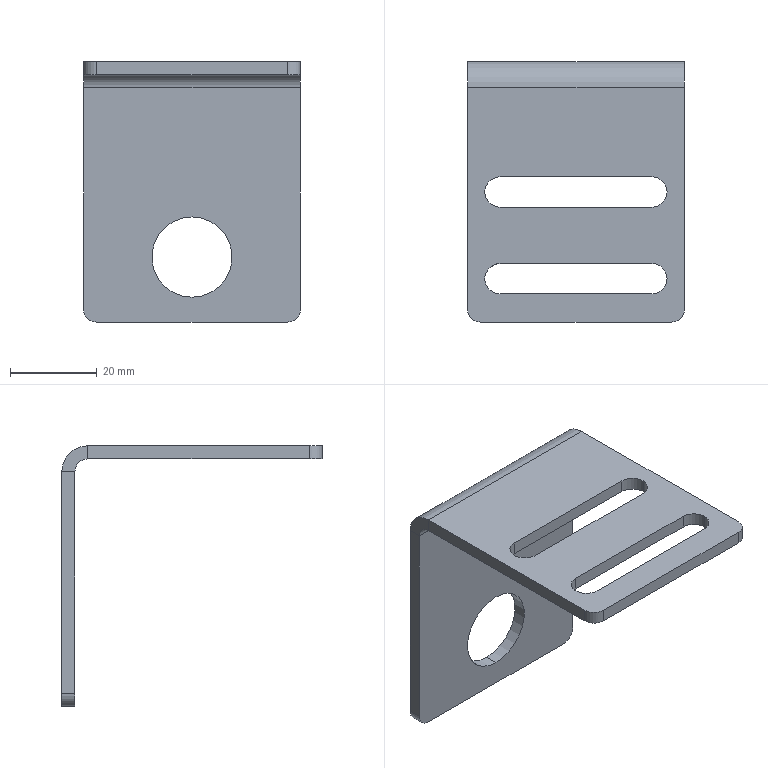Part | SolidWorks | features ICE 2, EdgeFlange 1, Fillet 1, FlatPattern 1, SMBaseFlange 1, SheetMetal 1 | 1 solid | 30 faces | box 50 x 60 x 60 mm | volume 14730 mm3 | plane 16 | cylinder 14 | commonest cylinder face diameters 7 x6 6 x5 18.5 x2 12 x1
STEP:
#1=CARTESIAN_POINT('',(0.,27.,-54.25));
#2=VERTEX_POINT('',#1);
#3=CARTESIAN_POINT('',(0.,27.,-35.75));
#4=VERTEX_POINT('',#3);
#5=CARTESIAN_POINT('',(0.,27.,-45.));
#6=DIRECTION('',(0.,1.,0.));
#7=DIRECTION('',(0.,0.,1.));
#8=AXIS2_PLACEMENT_3D('',#5,#6,#7);
#9=CIRCLE('',#8,9.25);
#10=EDGE_CURVE('',#2,#4,#9,.T.);
#11=ORIENTED_EDGE('',*,*,#10,.F.);
#12=CARTESIAN_POINT('',(0.,30.,-54.25));
#13=VERTEX_POINT('',#12);
#14=CARTESIAN_POINT('',(0.,20.,-54.25));
#15=DIRECTION('',(0.,1.,0.));
#16=VECTOR('',#15,1000.);
#17=LINE('',#14,#16);
#18=EDGE_CURVE('',#2,#13,#17,.T.);
#19=ORIENTED_EDGE('',*,*,#18,.T.);
#20=CARTESIAN_POINT('',(0.,30.,-35.75));
#21=VERTEX_POINT('',#20);
#22=CARTESIAN_POINT('',(0.,30.,-45.));
#23=DIRECTION('',(0.,1.,0.));
#24=DIRECTION('',(0.,0.,1.));
#25=AXIS2_PLACEMENT_3D('',#22,#23,#24);
#26=CIRCLE('',#25,9.25);
#27=EDGE_CURVE('',#13,#21,#26,.T.);
#28=ORIENTED_EDGE('',*,*,#27,.T.);
#29=CARTESIAN_POINT('',(0.,20.,-35.75));
#30=DIRECTION('',(0.,1.,0.));
#31=VECTOR('',#30,1000.);
#32=LINE('',#29,#31);
#33=EDGE_CURVE('',#4,#21,#32,.T.);
#34=ORIENTED_EDGE('',*,*,#33,.F.);
#35=EDGE_LOOP('',(#11,#19,#28,#34));
#36=FACE_OUTER_BOUND('',#35,.T.);
#37=CARTESIAN_POINT('',(0.,20.,-45.));
#38=DIRECTION('',(0.,1.,0.));
#39=DIRECTION('',(0.,0.,1.));
#40=AXIS2_PLACEMENT_3D('',#37,#38,#39);
#41=CYLINDRICAL_SURFACE('',#40,9.25);
#42=ADVANCED_FACE('',(#36),#41,.F.);
#43=CARTESIAN_POINT('',(21.,-20.,-3.));
#44=VERTEX_POINT('',#43);
#45=CARTESIAN_POINT('',(17.5,-16.5,-3.));
#46=VERTEX_POINT('',#45);
#47=CARTESIAN_POINT('',(17.5,-20.,-3.));
#48=DIRECTION('',(0.,0.,1.));
#49=DIRECTION('',(1.,0.,0.));
#50=AXIS2_PLACEMENT_3D('',#47,#48,#49);
#51=CIRCLE('',#50,3.5);
#52=EDGE_CURVE('',#44,#46,#51,.T.);
#53=ORIENTED_EDGE('',*,*,#52,.F.);
#54=CARTESIAN_POINT('',(21.,-20.,0.));
#55=VERTEX_POINT('',#54);
#56=CARTESIAN_POINT('',(21.,-20.,-10.));
#57=DIRECTION('',(0.,0.,1.));
#58=VECTOR('',#57,1000.);
#59=LINE('',#56,#58);
#60=EDGE_CURVE('',#44,#55,#59,.T.);
#61=ORIENTED_EDGE('',*,*,#60,.T.);
#62=CARTESIAN_POINT('',(17.5,-16.5,0.));
#63=VERTEX_POINT('',#62);
#64=CARTESIAN_POINT('',(17.5,-20.,0.));
#65=DIRECTION('',(0.,0.,1.));
#66=DIRECTION('',(1.,0.,0.));
#67=AXIS2_PLACEMENT_3D('',#64,#65,#66);
#68=CIRCLE('',#67,3.5);
#69=EDGE_CURVE('',#55,#63,#68,.T.);
#70=ORIENTED_EDGE('',*,*,#69,.T.);
#71=CARTESIAN_POINT('',(17.5,-16.5,-10.));
#72=DIRECTION('',(0.,0.,1.));
#73=VECTOR('',#72,1000.);
#74=LINE('',#71,#73);
#75=EDGE_CURVE('',#46,#63,#74,.T.);
#76=ORIENTED_EDGE('',*,*,#75,.F.);
#77=EDGE_LOOP('',(#53,#61,#70,#76));
#78=FACE_OUTER_BOUND('',#77,.T.);
#79=CARTESIAN_POINT('',(17.5,-20.,-10.));
#80=DIRECTION('',(0.,0.,1.));
#81=DIRECTION('',(1.,0.,0.));
#82=AXIS2_PLACEMENT_3D('',#79,#80,#81);
#83=CYLINDRICAL_SURFACE('',#82,3.5);
#84=ADVANCED_FACE('',(#78),#83,.F.);
#85=CARTESIAN_POINT('',(21.,0.,-3.));
#86=VERTEX_POINT('',#85);
#87=CARTESIAN_POINT('',(17.5,3.5,-3.));
#88=VERTEX_POINT('',#87);
#89=CARTESIAN_POINT('',(17.5,0.,-3.));
#90=DIRECTION('',(0.,0.,1.));
#91=DIRECTION('',(1.,0.,0.));
#92=AXIS2_PLACEMENT_3D('',#89,#90,#91);
#93=CIRCLE('',#92,3.5);
#94=EDGE_CURVE('',#86,#88,#93,.T.);
#95=ORIENTED_EDGE('',*,*,#94,.F.);
#96=CARTESIAN_POINT('',(21.,0.,0.));
#97=VERTEX_POINT('',#96);
#98=CARTESIAN_POINT('',(21.,0.,-10.));
#99=DIRECTION('',(0.,0.,1.));
#100=VECTOR('',#99,1000.);
#101=LINE('',#98,#100);
#102=EDGE_CURVE('',#86,#97,#101,.T.);
#103=ORIENTED_EDGE('',*,*,#102,.T.);
#104=CARTESIAN_POINT('',(17.5,3.5,0.));
#105=VERTEX_POINT('',#104);
#106=CARTESIAN_POINT('',(17.5,0.,0.));
#107=DIRECTION('',(0.,0.,1.));
#108=DIRECTION('',(1.,0.,0.));
#109=AXIS2_PLACEMENT_3D('',#106,#107,#108);
#110=CIRCLE('',#109,3.5);
#111=EDGE_CURVE('',#97,#105,#110,.T.);
#112=ORIENTED_EDGE('',*,*,#111,.T.);
#113=CARTESIAN_POINT('',(17.5,3.5,-10.));
#114=DIRECTION('',(0.,0.,1.));
#115=VECTOR('',#114,1000.);
#116=LINE('',#113,#115);
#117=EDGE_CURVE('',#88,#105,#116,.T.);
#118=ORIENTED_EDGE('',*,*,#117,.F.);
#119=EDGE_LOOP('',(#95,#103,#112,#118));
#120=FACE_OUTER_BOUND('',#119,.T.);
#121=CARTESIAN_POINT('',(17.5,0.,-10.));
#122=DIRECTION('',(0.,0.,1.));
#123=DIRECTION('',(1.,0.,0.));
#124=AXIS2_PLACEMENT_3D('',#121,#122,#123);
#125=CYLINDRICAL_SURFACE('',#124,3.5);
#126=ADVANCED_FACE('',(#120),#125,.F.);
#127=CARTESIAN_POINT('',(25.,-27.,0.));
#128=VERTEX_POINT('',#127);
#129=CARTESIAN_POINT('',(25.,24.,0.));
#130=VERTEX_POINT('',#129);
#131=CARTESIAN_POINT('',(25.,30.,0.));
#132=DIRECTION('',(0.,1.,0.));
#133=VECTOR('',#132,1000.);
#134=LINE('',#131,#133);
#135=EDGE_CURVE('',#128,#130,#134,.T.);
#136=ORIENTED_EDGE('',*,*,#135,.F.);
#137=CARTESIAN_POINT('',(25.,-27.,-3.));
#138=VERTEX_POINT('',#137);
#139=CARTESIAN_POINT('',(25.,-27.,-3.));
#140=DIRECTION('',(0.,0.,-1.));
#141=VECTOR('',#140,1000.);
#142=LINE('',#139,#141);
#143=EDGE_CURVE('',#128,#138,#142,.T.);
#144=ORIENTED_EDGE('',*,*,#143,.T.);
#145=CARTESIAN_POINT('',(25.,24.,-3.));
#146=VERTEX_POINT('',#145);
#147=CARTESIAN_POINT('',(25.,30.,-3.));
#148=DIRECTION('',(0.,1.,0.));
#149=VECTOR('',#148,1000.);
#150=LINE('',#147,#149);
#151=EDGE_CURVE('',#138,#146,#150,.T.);
#152=ORIENTED_EDGE('',*,*,#151,.T.);
#153=CARTESIAN_POINT('',(25.,24.,-3.));
#154=DIRECTION('',(0.,0.,1.));
#155=VECTOR('',#154,1000.);
#156=LINE('',#153,#155);
#157=EDGE_CURVE('',#146,#130,#156,.T.);
#158=ORIENTED_EDGE('',*,*,#157,.T.);
#159=EDGE_LOOP('',(#136,#144,#152,#158));
#160=FACE_OUTER_BOUND('',#159,.T.);
#161=CARTESIAN_POINT('',(25.,30.,-3.));
#162=DIRECTION('',(1.,0.,0.));
#163=DIRECTION('',(0.,1.,0.));
#164=AXIS2_PLACEMENT_3D('',#161,#162,#163);
#165=PLANE('',#164);
#166=ADVANCED_FACE('',(#160),#165,.T.);
#167=CARTESIAN_POINT('',(-17.5,-23.5,-3.));
#168=VERTEX_POINT('',#167);
#169=CARTESIAN_POINT('',(17.5,-23.5,-3.));
#170=VERTEX_POINT('',#169);
#171=CARTESIAN_POINT('',(0.,-23.5,-3.));
#172=DIRECTION('',(1.,0.,0.));
#173=VECTOR('',#172,1000.);
#174=LINE('',#171,#173);
#175=EDGE_CURVE('',#168,#170,#174,.T.);
#176=ORIENTED_EDGE('',*,*,#175,.T.);
#177=CARTESIAN_POINT('',(17.5,-20.,-3.));
#178=DIRECTION('',(0.,0.,1.));
#179=DIRECTION('',(1.,0.,0.));
#180=AXIS2_PLACEMENT_3D('',#177,#178,#179);
#181=CIRCLE('',#180,3.5);
#182=EDGE_CURVE('',#170,#44,#181,.T.);
#183=ORIENTED_EDGE('',*,*,#182,.T.);
#184=ORIENTED_EDGE('',*,*,#52,.T.);
#185=CARTESIAN_POINT('',(-17.5,-16.5,-3.));
#186=VERTEX_POINT('',#185);
#187=CARTESIAN_POINT('',(0.,-16.5,-3.));
#188=DIRECTION('',(-1.,0.,0.));
#189=VECTOR('',#188,1000.);
#190=LINE('',#187,#189);
#191=EDGE_CURVE('',#46,#186,#190,.T.);
#192=ORIENTED_EDGE('',*,*,#191,.T.);
#193=CARTESIAN_POINT('',(-17.5,-20.,-3.));
#194=DIRECTION('',(0.,0.,1.));
#195=DIRECTION('',(1.,0.,0.));
#196=AXIS2_PLACEMENT_3D('',#193,#194,#195);
#197=CIRCLE('',#196,3.5);
#198=EDGE_CURVE('',#186,#168,#197,.T.);
#199=ORIENTED_EDGE('',*,*,#198,.T.);
#200=EDGE_LOOP('',(#176,#183,#184,#192,#199));
#201=FACE_BOUND('',#200,.T.);
#202=CARTESIAN_POINT('',(-17.5,-3.5,-3.));
#203=VERTEX_POINT('',#202);
#204=CARTESIAN_POINT('',(17.5,-3.5,-3.));
#205=VERTEX_POINT('',#204);
#206=CARTESIAN_POINT('',(0.,-3.5,-3.));
#207=DIRECTION('',(1.,0.,0.));
#208=VECTOR('',#207,1000.);
#209=LINE('',#206,#208);
#210=EDGE_CURVE('',#203,#205,#209,.T.);
#211=ORIENTED_EDGE('',*,*,#210,.T.);
#212=CARTESIAN_POINT('',(17.5,0.,-3.));
#213=DIRECTION('',(0.,0.,1.));
#214=DIRECTION('',(1.,0.,0.));
#215=AXIS2_PLACEMENT_3D('',#212,#213,#214);
#216=CIRCLE('',#215,3.5);
#217=EDGE_CURVE('',#205,#86,#216,.T.);
#218=ORIENTED_EDGE('',*,*,#217,.T.);
#219=ORIENTED_EDGE('',*,*,#94,.T.);
#220=CARTESIAN_POINT('',(-17.5,3.5,-3.));
#221=VERTEX_POINT('',#220);
#222=CARTESIAN_POINT('',(0.,3.5,-3.));
#223=DIRECTION('',(-1.,0.,0.));
#224=VECTOR('',#223,1000.);
#225=LINE('',#222,#224);
#226=EDGE_CURVE('',#88,#221,#225,.T.);
#227=ORIENTED_EDGE('',*,*,#226,.T.);
#228=CARTESIAN_POINT('',(-17.5,0.,-3.));
#229=DIRECTION('',(0.,0.,1.));
#230=DIRECTION('',(1.,0.,0.));
#231=AXIS2_PLACEMENT_3D('',#228,#229,#230);
#232=CIRCLE('',#231,3.5);
#233=EDGE_CURVE('',#221,#203,#232,.T.);
#234=ORIENTED_EDGE('',*,*,#233,.T.);
#235=EDGE_LOOP('',(#211,#218,#219,#227,#234));
#236=FACE_BOUND('',#235,.T.);
#237=ORIENTED_EDGE('',*,*,#151,.F.);
#238=CARTESIAN_POINT('',(22.,-30.,-3.));
#239=VERTEX_POINT('',#238);
#240=CARTESIAN_POINT('',(22.,-27.,-3.));
#241=DIRECTION('',(0.,0.,-1.));
#242=DIRECTION('',(1.,0.,0.));
#243=AXIS2_PLACEMENT_3D('',#240,#241,#242);
#244=CIRCLE('',#243,3.);
#245=EDGE_CURVE('',#138,#239,#244,.T.);
#246=ORIENTED_EDGE('',*,*,#245,.T.);
#247=CARTESIAN_POINT('',(-22.,-30.,-3.));
#248=VERTEX_POINT('',#247);
#249=CARTESIAN_POINT('',(-25.,-30.,-3.));
#250=DIRECTION('',(1.,0.,0.));
#251=VECTOR('',#250,1000.);
#252=LINE('',#249,#251);
#253=EDGE_CURVE('',#248,#239,#252,.T.);
#254=ORIENTED_EDGE('',*,*,#253,.F.);
#255=CARTESIAN_POINT('',(-25.,-27.,-3.));
#256=VERTEX_POINT('',#255);
#257=CARTESIAN_POINT('',(-22.,-27.,-3.));
#258=DIRECTION('',(0.,0.,-1.));
#259=DIRECTION('',(1.,0.,0.));
#260=AXIS2_PLACEMENT_3D('',#257,#258,#259);
#261=CIRCLE('',#260,3.);
#262=EDGE_CURVE('',#248,#256,#261,.T.);
#263=ORIENTED_EDGE('',*,*,#262,.T.);
#264=CARTESIAN_POINT('',(-25.,24.,-3.));
#265=VERTEX_POINT('',#264);
#266=CARTESIAN_POINT('',(-25.,30.,-3.));
#267=DIRECTION('',(0.,-1.,0.));
#268=VECTOR('',#267,1000.);
#269=LINE('',#266,#268);
#270=EDGE_CURVE('',#265,#256,#269,.T.);
#271=ORIENTED_EDGE('',*,*,#270,.F.);
#272=CARTESIAN_POINT('',(25.,24.,-3.));
#273=DIRECTION('',(-1.,0.,0.));
#274=VECTOR('',#273,1000.);
#275=LINE('',#272,#274);
#276=EDGE_CURVE('',#146,#265,#275,.T.);
#277=ORIENTED_EDGE('',*,*,#276,.F.);
#278=EDGE_LOOP('',(#237,#246,#254,#263,#271,#277));
#279=FACE_OUTER_BOUND('',#278,.T.);
#280=CARTESIAN_POINT('',(0.,0.,-3.));
#281=DIRECTION('',(0.,0.,1.));
#282=DIRECTION('',(1.,0.,0.));
#283=AXIS2_PLACEMENT_3D('',#280,#281,#282);
#284=PLANE('',#283);
#285=ADVANCED_FACE('',(#201,#236,#279),#284,.F.);
#286=CARTESIAN_POINT('',(17.5,-23.5,0.));
#287=VERTEX_POINT('',#286);
#288=CARTESIAN_POINT('',(17.5,-20.,0.));
#289=DIRECTION('',(0.,0.,1.));
#290=DIRECTION('',(1.,0.,0.));
#291=AXIS2_PLACEMENT_3D('',#288,#289,#290);
#292=CIRCLE('',#291,3.5);
#293=EDGE_CURVE('',#287,#55,#292,.T.);
#294=ORIENTED_EDGE('',*,*,#293,.F.);
#295=CARTESIAN_POINT('',(-17.5,-23.5,0.));
#296=VERTEX_POINT('',#295);
#297=CARTESIAN_POINT('',(-17.5,-23.5,0.));
#298=DIRECTION('',(1.,0.,0.));
#299=VECTOR('',#298,1000.);
#300=LINE('',#297,#299);
#301=EDGE_CURVE('',#296,#287,#300,.T.);
#302=ORIENTED_EDGE('',*,*,#301,.F.);
#303=CARTESIAN_POINT('',(-17.5,-16.5,0.));
#304=VERTEX_POINT('',#303);
#305=CARTESIAN_POINT('',(-17.5,-20.,0.));
#306=DIRECTION('',(0.,0.,1.));
#307=DIRECTION('',(1.,0.,0.));
#308=AXIS2_PLACEMENT_3D('',#305,#306,#307);
#309=CIRCLE('',#308,3.5);
#310=EDGE_CURVE('',#304,#296,#309,.T.);
#311=ORIENTED_EDGE('',*,*,#310,.F.);
#312=CARTESIAN_POINT('',(-17.5,-16.5,0.));
#313=DIRECTION('',(-1.,0.,0.));
#314=VECTOR('',#313,1000.);
#315=LINE('',#312,#314);
#316=EDGE_CURVE('',#63,#304,#315,.T.);
#317=ORIENTED_EDGE('',*,*,#316,.F.);
#318=ORIENTED_EDGE('',*,*,#69,.F.);
#319=EDGE_LOOP('',(#294,#302,#311,#317,#318));
#320=FACE_BOUND('',#319,.T.);
#321=CARTESIAN_POINT('',(17.5,-3.5,0.));
#322=VERTEX_POINT('',#321);
#323=CARTESIAN_POINT('',(17.5,0.,0.));
#324=DIRECTION('',(0.,0.,1.));
#325=DIRECTION('',(1.,0.,0.));
#326=AXIS2_PLACEMENT_3D('',#323,#324,#325);
#327=CIRCLE('',#326,3.5);
#328=EDGE_CURVE('',#322,#97,#327,.T.);
#329=ORIENTED_EDGE('',*,*,#328,.F.);
#330=CARTESIAN_POINT('',(-17.5,-3.5,0.));
#331=VERTEX_POINT('',#330);
#332=CARTESIAN_POINT('',(-17.5,-3.5,0.));
#333=DIRECTION('',(1.,0.,0.));
#334=VECTOR('',#333,1000.);
#335=LINE('',#332,#334);
#336=EDGE_CURVE('',#331,#322,#335,.T.);
#337=ORIENTED_EDGE('',*,*,#336,.F.);
#338=CARTESIAN_POINT('',(-17.5,3.5,0.));
#339=VERTEX_POINT('',#338);
#340=CARTESIAN_POINT('',(-17.5,0.,0.));
#341=DIRECTION('',(0.,0.,1.));
#342=DIRECTION('',(1.,0.,0.));
#343=AXIS2_PLACEMENT_3D('',#340,#341,#342);
#344=CIRCLE('',#343,3.5);
#345=EDGE_CURVE('',#339,#331,#344,.T.);
#346=ORIENTED_EDGE('',*,*,#345,.F.);
#347=CARTESIAN_POINT('',(-17.5,3.5,0.));
#348=DIRECTION('',(-1.,0.,0.));
#349=VECTOR('',#348,1000.);
#350=LINE('',#347,#349);
#351=EDGE_CURVE('',#105,#339,#350,.T.);
#352=ORIENTED_EDGE('',*,*,#351,.F.);
#353=ORIENTED_EDGE('',*,*,#111,.F.);
#354=EDGE_LOOP('',(#329,#337,#346,#352,#353));
#355=FACE_BOUND('',#354,.T.);
#356=CARTESIAN_POINT('',(-22.,-30.,0.));
#357=VERTEX_POINT('',#356);
#358=CARTESIAN_POINT('',(22.,-30.,0.));
#359=VERTEX_POINT('',#358);
#360=CARTESIAN_POINT('',(-25.,-30.,0.));
#361=DIRECTION('',(1.,0.,0.));
#362=VECTOR('',#361,1000.);
#363=LINE('',#360,#362);
#364=EDGE_CURVE('',#357,#359,#363,.T.);
#365=ORIENTED_EDGE('',*,*,#364,.T.);
#366=CARTESIAN_POINT('',(22.,-27.,0.));
#367=DIRECTION('',(0.,0.,1.));
#368=DIRECTION('',(1.,0.,0.));
#369=AXIS2_PLACEMENT_3D('',#366,#367,#368);
#370=CIRCLE('',#369,3.);
#371=EDGE_CURVE('',#359,#128,#370,.T.);
#372=ORIENTED_EDGE('',*,*,#371,.T.);
#373=ORIENTED_EDGE('',*,*,#135,.T.);
#374=CARTESIAN_POINT('',(-25.,24.,0.));
#375=VERTEX_POINT('',#374);
#376=CARTESIAN_POINT('',(25.,24.,0.));
#377=DIRECTION('',(-1.,0.,0.));
#378=VECTOR('',#377,1000.);
#379=LINE('',#376,#378);
#380=EDGE_CURVE('',#130,#375,#379,.T.);
#381=ORIENTED_EDGE('',*,*,#380,.T.);
#382=CARTESIAN_POINT('',(-25.,-27.,0.));
#383=VERTEX_POINT('',#382);
#384=CARTESIAN_POINT('',(-25.,30.,0.));
#385=DIRECTION('',(0.,-1.,0.));
#386=VECTOR('',#385,1000.);
#387=LINE('',#384,#386);
#388=EDGE_CURVE('',#375,#383,#387,.T.);
#389=ORIENTED_EDGE('',*,*,#388,.T.);
#390=CARTESIAN_POINT('',(-22.,-27.,0.));
#391=DIRECTION('',(0.,0.,1.));
#392=DIRECTION('',(1.,0.,0.));
#393=AXIS2_PLACEMENT_3D('',#390,#391,#392);
#394=CIRCLE('',#393,3.);
#395=EDGE_CURVE('',#383,#357,#394,.T.);
#396=ORIENTED_EDGE('',*,*,#395,.T.);
#397=EDGE_LOOP('',(#365,#372,#373,#381,#389,#396));
#398=FACE_OUTER_BOUND('',#397,.T.);
#399=CARTESIAN_POINT('',(0.,0.,0.));
#400=DIRECTION('',(0.,0.,1.));
#401=DIRECTION('',(1.,0.,0.));
#402=AXIS2_PLACEMENT_3D('',#399,#400,#401);
#403=PLANE('',#402);
#404=ADVANCED_FACE('',(#320,#355,#398),#403,.T.);
#405=ORIENTED_EDGE('',*,*,#253,.T.);
#406=CARTESIAN_POINT('',(22.,-30.,-3.));
#407=DIRECTION('',(0.,0.,1.));
#408=VECTOR('',#407,1000.);
#409=LINE('',#406,#408);
#410=EDGE_CURVE('',#239,#359,#409,.T.);
#411=ORIENTED_EDGE('',*,*,#410,.T.);
#412=ORIENTED_EDGE('',*,*,#364,.F.);
#413=CARTESIAN_POINT('',(-22.,-30.,-3.));
#414=DIRECTION('',(0.,0.,-1.));
#415=VECTOR('',#414,1000.);
#416=LINE('',#413,#415);
#417=EDGE_CURVE('',#357,#248,#416,.T.);
#418=ORIENTED_EDGE('',*,*,#417,.T.);
#419=EDGE_LOOP('',(#405,#411,#412,#418));
#420=FACE_OUTER_BOUND('',#419,.T.);
#421=CARTESIAN_POINT('',(-25.,-30.,-3.));
#422=DIRECTION('',(0.,-1.,0.));
#423=DIRECTION('',(0.,0.,-1.));
#424=AXIS2_PLACEMENT_3D('',#421,#422,#423);
#425=PLANE('',#424);
#426=ADVANCED_FACE('',(#420),#425,.T.);
#427=ORIENTED_EDGE('',*,*,#270,.T.);
#428=CARTESIAN_POINT('',(-25.,-27.,-3.));
#429=DIRECTION('',(0.,0.,1.));
#430=VECTOR('',#429,1000.);
#431=LINE('',#428,#430);
#432=EDGE_CURVE('',#256,#383,#431,.T.);
#433=ORIENTED_EDGE('',*,*,#432,.T.);
#434=ORIENTED_EDGE('',*,*,#388,.F.);
#435=CARTESIAN_POINT('',(-25.,24.,-3.));
#436=DIRECTION('',(0.,0.,1.));
#437=VECTOR('',#436,1000.);
#438=LINE('',#435,#437);
#439=EDGE_CURVE('',#265,#375,#438,.T.);
#440=ORIENTED_EDGE('',*,*,#439,.F.);
#441=EDGE_LOOP('',(#427,#433,#434,#440));
#442=FACE_OUTER_BOUND('',#441,.T.);
#443=CARTESIAN_POINT('',(-25.,30.,-3.));
#444=DIRECTION('',(-1.,0.,0.));
#445=DIRECTION('',(0.,-1.,0.));
#446=AXIS2_PLACEMENT_3D('',#443,#444,#445);
#447=PLANE('',#446);
#448=ADVANCED_FACE('',(#442),#447,.T.);
#449=CARTESIAN_POINT('',(-25.,27.,-6.));
#450=VERTEX_POINT('',#449);
#451=CARTESIAN_POINT('',(-25.,30.,-6.));
#452=VERTEX_POINT('',#451);
#453=CARTESIAN_POINT('',(-25.,30.,-6.));
#454=DIRECTION('',(0.,1.,0.));
#455=VECTOR('',#454,1000.);
#456=LINE('',#453,#455);
#457=EDGE_CURVE('',#450,#452,#456,.T.);
#458=ORIENTED_EDGE('',*,*,#457,.F.);
#459=CARTESIAN_POINT('',(-25.,24.,-6.));
#460=DIRECTION('',(-1.,0.,0.));
#461=DIRECTION('',(0.,0.,-1.));
#462=AXIS2_PLACEMENT_3D('',#459,#460,#461);
#463=CIRCLE('',#462,3.);
#464=EDGE_CURVE('',#265,#450,#463,.T.);
#465=ORIENTED_EDGE('',*,*,#464,.F.);
#466=ORIENTED_EDGE('',*,*,#439,.T.);
#467=CARTESIAN_POINT('',(-25.,24.,-6.));
#468=DIRECTION('',(-1.,0.,0.));
#469=DIRECTION('',(0.,0.,-1.));
#470=AXIS2_PLACEMENT_3D('',#467,#468,#469);
#471=CIRCLE('',#470,6.);
#472=EDGE_CURVE('',#375,#452,#471,.T.);
#473=ORIENTED_EDGE('',*,*,#472,.T.);
#474=EDGE_LOOP('',(#458,#465,#466,#473));
#475=FACE_OUTER_BOUND('',#474,.T.);
#476=CARTESIAN_POINT('',(-25.,24.,-6.));
#477=DIRECTION('',(-1.,0.,0.));
#478=DIRECTION('',(0.,0.,1.));
#479=AXIS2_PLACEMENT_3D('',#476,#477,#478);
#480=PLANE('',#479);
#481=ADVANCED_FACE('',(#475),#480,.T.);
#482=CARTESIAN_POINT('',(25.,27.,-6.));
#483=VERTEX_POINT('',#482);
#484=CARTESIAN_POINT('',(25.,24.,-6.));
#485=DIRECTION('',(1.,0.,0.));
#486=DIRECTION('',(0.,0.,-1.));
#487=AXIS2_PLACEMENT_3D('',#484,#485,#486);
#488=CIRCLE('',#487,3.);
#489=EDGE_CURVE('',#483,#146,#488,.T.);
#490=ORIENTED_EDGE('',*,*,#489,.F.);
#491=CARTESIAN_POINT('',(25.,30.,-6.));
#492=VERTEX_POINT('',#491);
#493=CARTESIAN_POINT('',(25.,27.,-6.));
#494=DIRECTION('',(0.,1.,0.));
#495=VECTOR('',#494,1000.);
#496=LINE('',#493,#495);
#497=EDGE_CURVE('',#483,#492,#496,.T.);
#498=ORIENTED_EDGE('',*,*,#497,.T.);
#499=CARTESIAN_POINT('',(25.,24.,-6.));
#500=DIRECTION('',(1.,0.,0.));
#501=DIRECTION('',(0.,0.,-1.));
#502=AXIS2_PLACEMENT_3D('',#499,#500,#501);
#503=CIRCLE('',#502,6.);
#504=EDGE_CURVE('',#492,#130,#503,.T.);
#505=ORIENTED_EDGE('',*,*,#504,.T.);
#506=ORIENTED_EDGE('',*,*,#157,.F.);
#507=EDGE_LOOP('',(#490,#498,#505,#506));
#508=FACE_OUTER_BOUND('',#507,.T.);
#509=CARTESIAN_POINT('',(25.,24.,-6.));
#510=DIRECTION('',(-1.,0.,0.));
#511=DIRECTION('',(0.,0.,1.));
#512=AXIS2_PLACEMENT_3D('',#509,#510,#511);
#513=PLANE('',#512);
#514=ADVANCED_FACE('',(#508),#513,.F.);
#515=ORIENTED_EDGE('',*,*,#380,.F.);
#516=ORIENTED_EDGE('',*,*,#504,.F.);
#517=CARTESIAN_POINT('',(0.,30.,-6.));
#518=DIRECTION('',(1.,0.,0.));
#519=VECTOR('',#518,1000.);
#520=LINE('',#517,#519);
#521=EDGE_CURVE('',#452,#492,#520,.T.);
#522=ORIENTED_EDGE('',*,*,#521,.F.);
#523=ORIENTED_EDGE('',*,*,#472,.F.);
#524=EDGE_LOOP('',(#515,#516,#522,#523));
#525=FACE_OUTER_BOUND('',#524,.T.);
#526=CARTESIAN_POINT('',(25.,24.,-6.));
#527=DIRECTION('',(1.,0.,0.));
#528=DIRECTION('',(0.,1.,0.));
#529=AXIS2_PLACEMENT_3D('',#526,#527,#528);
#530=CYLINDRICAL_SURFACE('',#529,6.);
#531=ADVANCED_FACE('',(#525),#530,.T.);
#532=ORIENTED_EDGE('',*,*,#276,.T.);
#533=ORIENTED_EDGE('',*,*,#464,.T.);
#534=CARTESIAN_POINT('',(-25.,27.,-6.));
#535=DIRECTION('',(1.,0.,0.));
#536=VECTOR('',#535,1000.);
#537=LINE('',#534,#536);
#538=EDGE_CURVE('',#450,#483,#537,.T.);
#539=ORIENTED_EDGE('',*,*,#538,.T.);
#540=ORIENTED_EDGE('',*,*,#489,.T.);
#541=EDGE_LOOP('',(#532,#533,#539,#540));
#542=FACE_OUTER_BOUND('',#541,.T.);
#543=CARTESIAN_POINT('',(25.,24.,-6.));
#544=DIRECTION('',(1.,0.,0.));
#545=DIRECTION('',(0.,1.,0.));
#546=AXIS2_PLACEMENT_3D('',#543,#544,#545);
#547=CYLINDRICAL_SURFACE('',#546,3.);
#548=ADVANCED_FACE('',(#542),#547,.F.);
#549=CARTESIAN_POINT('',(25.,27.,-57.));
#550=VERTEX_POINT('',#549);
#551=CARTESIAN_POINT('',(25.,27.,0.));
#552=DIRECTION('',(0.,0.,1.));
#553=VECTOR('',#552,1000.);
#554=LINE('',#551,#553);
#555=EDGE_CURVE('',#550,#483,#554,.T.);
#556=ORIENTED_EDGE('',*,*,#555,.F.);
#557=CARTESIAN_POINT('',(25.,30.,-57.));
#558=VERTEX_POINT('',#557);
#559=CARTESIAN_POINT('',(25.,30.,-57.));
#560=DIRECTION('',(0.,1.,0.));
#561=VECTOR('',#560,1000.);
#562=LINE('',#559,#561);
#563=EDGE_CURVE('',#550,#558,#562,.T.);
#564=ORIENTED_EDGE('',*,*,#563,.T.);
#565=CARTESIAN_POINT('',(25.,30.,-3.));
#566=DIRECTION('',(0.,0.,1.));
#567=VECTOR('',#566,1000.);
#568=LINE('',#565,#567);
#569=EDGE_CURVE('',#558,#492,#568,.T.);
#570=ORIENTED_EDGE('',*,*,#569,.T.);
#571=ORIENTED_EDGE('',*,*,#497,.F.);
#572=EDGE_LOOP('',(#556,#564,#570,#571));
#573=FACE_OUTER_BOUND('',#572,.T.);
#574=CARTESIAN_POINT('',(25.,30.,-3.));
#575=DIRECTION('',(1.,0.,0.));
#576=DIRECTION('',(0.,0.,-1.));
#577=AXIS2_PLACEMENT_3D('',#574,#575,#576);
#578=PLANE('',#577);
#579=ADVANCED_FACE('',(#573),#578,.T.);
#580=CARTESIAN_POINT('',(-25.,30.,-57.));
#581=VERTEX_POINT('',#580);
#582=CARTESIAN_POINT('',(-25.,30.,-60.));
#583=DIRECTION('',(0.,0.,-1.));
#584=VECTOR('',#583,1000.);
#585=LINE('',#582,#584);
#586=EDGE_CURVE('',#452,#581,#585,.T.);
#587=ORIENTED_EDGE('',*,*,#586,.T.);
#588=CARTESIAN_POINT('',(-25.,27.,-57.));
#589=VERTEX_POINT('',#588);
#590=CARTESIAN_POINT('',(-25.,30.,-57.));
#591=DIRECTION('',(0.,-1.,0.));
#592=VECTOR('',#591,1000.);
#593=LINE('',#590,#592);
#594=EDGE_CURVE('',#581,#589,#593,.T.);
#595=ORIENTED_EDGE('',*,*,#594,.T.);
#596=CARTESIAN_POINT('',(-25.,27.,0.));
#597=DIRECTION('',(0.,0.,-1.));
#598=VECTOR('',#597,1000.);
#599=LINE('',#596,#598);
#600=EDGE_CURVE('',#450,#589,#599,.T.);
#601=ORIENTED_EDGE('',*,*,#600,.F.);
#602=ORIENTED_EDGE('',*,*,#457,.T.);
#603=EDGE_LOOP('',(#587,#595,#601,#602));
#604=FACE_OUTER_BOUND('',#603,.T.);
#605=CARTESIAN_POINT('',(-25.,30.,-60.));
#606=DIRECTION('',(-1.,0.,0.));
#607=DIRECTION('',(0.,0.,1.));
#608=AXIS2_PLACEMENT_3D('',#605,#606,#607);
#609=PLANE('',#608);
#610=ADVANCED_FACE('',(#604),#609,.T.);
#611=CARTESIAN_POINT('',(0.,30.,-45.));
#612=DIRECTION('',(0.,1.,0.));
#613=DIRECTION('',(0.,0.,1.));
#614=AXIS2_PLACEMENT_3D('',#611,#612,#613);
#615=CIRCLE('',#614,9.25);
#616=EDGE_CURVE('',#21,#13,#615,.T.);
#617=ORIENTED_EDGE('',*,*,#616,.F.);
#618=ORIENTED_EDGE('',*,*,#27,.F.);
#619=EDGE_LOOP('',(#617,#618));
#620=FACE_BOUND('',#619,.T.);
#621=CARTESIAN_POINT('',(-22.,30.,-60.));
#622=VERTEX_POINT('',#621);
#623=CARTESIAN_POINT('',(22.,30.,-60.));
#624=VERTEX_POINT('',#623);
#625=CARTESIAN_POINT('',(25.,30.,-60.));
#626=DIRECTION('',(1.,0.,0.));
#627=VECTOR('',#626,1000.);
#628=LINE('',#625,#627);
#629=EDGE_CURVE('',#622,#624,#628,.T.);
#630=ORIENTED_EDGE('',*,*,#629,.F.);
#631=CARTESIAN_POINT('',(-22.,30.,-57.));
#632=DIRECTION('',(0.,1.,0.));
#633=DIRECTION('',(0.,0.,1.));
#634=AXIS2_PLACEMENT_3D('',#631,#632,#633);
#635=CIRCLE('',#634,3.);
#636=EDGE_CURVE('',#622,#581,#635,.T.);
#637=ORIENTED_EDGE('',*,*,#636,.T.);
#638=ORIENTED_EDGE('',*,*,#586,.F.);
#639=ORIENTED_EDGE('',*,*,#521,.T.);
#640=ORIENTED_EDGE('',*,*,#569,.F.);
#641=CARTESIAN_POINT('',(22.,30.,-57.));
#642=DIRECTION('',(0.,1.,0.));
#643=DIRECTION('',(0.,0.,1.));
#644=AXIS2_PLACEMENT_3D('',#641,#642,#643);
#645=CIRCLE('',#644,3.);
#646=EDGE_CURVE('',#558,#624,#645,.T.);
#647=ORIENTED_EDGE('',*,*,#646,.T.);
#648=EDGE_LOOP('',(#630,#637,#638,#639,#640,#647));
#649=FACE_OUTER_BOUND('',#648,.T.);
#650=CARTESIAN_POINT('',(0.,30.,0.));
#651=DIRECTION('',(0.,1.,0.));
#652=DIRECTION('',(0.,0.,1.));
#653=AXIS2_PLACEMENT_3D('',#650,#651,#652);
#654=PLANE('',#653);
#655=ADVANCED_FACE('',(#620,#649),#654,.T.);
#656=CARTESIAN_POINT('',(0.,27.,-45.));
#657=DIRECTION('',(0.,1.,0.));
#658=DIRECTION('',(0.,0.,1.));
#659=AXIS2_PLACEMENT_3D('',#656,#657,#658);
#660=CIRCLE('',#659,9.25);
#661=EDGE_CURVE('',#4,#2,#660,.T.);
#662=ORIENTED_EDGE('',*,*,#661,.T.);
#663=ORIENTED_EDGE('',*,*,#10,.T.);
#664=EDGE_LOOP('',(#662,#663));
#665=FACE_BOUND('',#664,.T.);
#666=ORIENTED_EDGE('',*,*,#600,.T.);
#667=CARTESIAN_POINT('',(-22.,27.,-60.));
#668=VERTEX_POINT('',#667);
#669=CARTESIAN_POINT('',(-22.,27.,-57.));
#670=DIRECTION('',(0.,-1.,0.));
#671=DIRECTION('',(0.,0.,1.));
#672=AXIS2_PLACEMENT_3D('',#669,#670,#671);
#673=CIRCLE('',#672,3.);
#674=EDGE_CURVE('',#589,#668,#673,.T.);
#675=ORIENTED_EDGE('',*,*,#674,.T.);
#676=CARTESIAN_POINT('',(22.,27.,-60.));
#677=VERTEX_POINT('',#676);
#678=CARTESIAN_POINT('',(0.,27.,-60.));
#679=DIRECTION('',(1.,0.,0.));
#680=VECTOR('',#679,1000.);
#681=LINE('',#678,#680);
#682=EDGE_CURVE('',#668,#677,#681,.T.);
#683=ORIENTED_EDGE('',*,*,#682,.T.);
#684=CARTESIAN_POINT('',(22.,27.,-57.));
#685=DIRECTION('',(0.,-1.,0.));
#686=DIRECTION('',(0.,0.,1.));
#687=AXIS2_PLACEMENT_3D('',#684,#685,#686);
#688=CIRCLE('',#687,3.);
#689=EDGE_CURVE('',#677,#550,#688,.T.);
#690=ORIENTED_EDGE('',*,*,#689,.T.);
#691=ORIENTED_EDGE('',*,*,#555,.T.);
#692=ORIENTED_EDGE('',*,*,#538,.F.);
#693=EDGE_LOOP('',(#666,#675,#683,#690,#691,#692));
#694=FACE_OUTER_BOUND('',#693,.T.);
#695=CARTESIAN_POINT('',(0.,27.,0.));
#696=DIRECTION('',(0.,1.,0.));
#697=DIRECTION('',(0.,0.,1.));
#698=AXIS2_PLACEMENT_3D('',#695,#696,#697);
#699=PLANE('',#698);
#700=ADVANCED_FACE('',(#665,#694),#699,.F.);
#701=ORIENTED_EDGE('',*,*,#682,.F.);
#702=CARTESIAN_POINT('',(-22.,30.,-60.));
#703=DIRECTION('',(0.,1.,0.));
#704=VECTOR('',#703,1000.);
#705=LINE('',#702,#704);
#706=EDGE_CURVE('',#668,#622,#705,.T.);
#707=ORIENTED_EDGE('',*,*,#706,.T.);
#708=ORIENTED_EDGE('',*,*,#629,.T.);
#709=CARTESIAN_POINT('',(22.,30.,-60.));
#710=DIRECTION('',(0.,-1.,0.));
#711=VECTOR('',#710,1000.);
#712=LINE('',#709,#711);
#713=EDGE_CURVE('',#624,#677,#712,.T.);
#714=ORIENTED_EDGE('',*,*,#713,.T.);
#715=EDGE_LOOP('',(#701,#707,#708,#714));
#716=FACE_OUTER_BOUND('',#715,.T.);
#717=CARTESIAN_POINT('',(25.,30.,-60.));
#718=DIRECTION('',(0.,0.,-1.));
#719=DIRECTION('',(0.,1.,0.));
#720=AXIS2_PLACEMENT_3D('',#717,#718,#719);
#721=PLANE('',#720);
#722=ADVANCED_FACE('',(#716),#721,.T.);
#723=ORIENTED_EDGE('',*,*,#102,.F.);
#724=ORIENTED_EDGE('',*,*,#217,.F.);
#725=CARTESIAN_POINT('',(17.5,-3.5,-10.));
#726=DIRECTION('',(0.,0.,1.));
#727=VECTOR('',#726,1000.);
#728=LINE('',#725,#727);
#729=EDGE_CURVE('',#205,#322,#728,.T.);
#730=ORIENTED_EDGE('',*,*,#729,.T.);
#731=ORIENTED_EDGE('',*,*,#328,.T.);
#732=EDGE_LOOP('',(#723,#724,#730,#731));
#733=FACE_OUTER_BOUND('',#732,.T.);
#734=CARTESIAN_POINT('',(17.5,0.,-10.));
#735=DIRECTION('',(0.,0.,1.));
#736=DIRECTION('',(1.,0.,0.));
#737=AXIS2_PLACEMENT_3D('',#734,#735,#736);
#738=CYLINDRICAL_SURFACE('',#737,3.5);
#739=ADVANCED_FACE('',(#733),#738,.F.);
#740=CARTESIAN_POINT('',(-17.5,-3.5,-10.));
#741=DIRECTION('',(0.,0.,1.));
#742=VECTOR('',#741,1000.);
#743=LINE('',#740,#742);
#744=EDGE_CURVE('',#203,#331,#743,.T.);
#745=ORIENTED_EDGE('',*,*,#744,.T.);
#746=ORIENTED_EDGE('',*,*,#336,.T.);
#747=ORIENTED_EDGE('',*,*,#729,.F.);
#748=ORIENTED_EDGE('',*,*,#210,.F.);
#749=EDGE_LOOP('',(#745,#746,#747,#748));
#750=FACE_OUTER_BOUND('',#749,.T.);
#751=CARTESIAN_POINT('',(-17.5,-3.5,-10.));
#752=DIRECTION('',(0.,-1.,0.));
#753=DIRECTION('',(0.,0.,-1.));
#754=AXIS2_PLACEMENT_3D('',#751,#752,#753);
#755=PLANE('',#754);
#756=ADVANCED_FACE('',(#750),#755,.F.);
#757=CARTESIAN_POINT('',(-17.5,3.5,-10.));
#758=DIRECTION('',(0.,0.,1.));
#759=VECTOR('',#758,1000.);
#760=LINE('',#757,#759);
#761=EDGE_CURVE('',#221,#339,#760,.T.);
#762=ORIENTED_EDGE('',*,*,#761,.T.);
#763=ORIENTED_EDGE('',*,*,#345,.T.);
#764=ORIENTED_EDGE('',*,*,#744,.F.);
#765=ORIENTED_EDGE('',*,*,#233,.F.);
#766=EDGE_LOOP('',(#762,#763,#764,#765));
#767=FACE_OUTER_BOUND('',#766,.T.);
#768=CARTESIAN_POINT('',(-17.5,0.,-10.));
#769=DIRECTION('',(0.,0.,1.));
#770=DIRECTION('',(1.,0.,0.));
#771=AXIS2_PLACEMENT_3D('',#768,#769,#770);
#772=CYLINDRICAL_SURFACE('',#771,3.5);
#773=ADVANCED_FACE('',(#767),#772,.F.);
#774=ORIENTED_EDGE('',*,*,#117,.T.);
#775=ORIENTED_EDGE('',*,*,#351,.T.);
#776=ORIENTED_EDGE('',*,*,#761,.F.);
#777=ORIENTED_EDGE('',*,*,#226,.F.);
#778=EDGE_LOOP('',(#774,#775,#776,#777));
#779=FACE_OUTER_BOUND('',#778,.T.);
#780=CARTESIAN_POINT('',(-17.5,3.5,-10.));
#781=DIRECTION('',(0.,1.,0.));
#782=DIRECTION('',(-1.,0.,0.));
#783=AXIS2_PLACEMENT_3D('',#780,#781,#782);
#784=PLANE('',#783);
#785=ADVANCED_FACE('',(#779),#784,.F.);
#786=ORIENTED_EDGE('',*,*,#60,.F.);
#787=ORIENTED_EDGE('',*,*,#182,.F.);
#788=CARTESIAN_POINT('',(17.5,-23.5,-10.));
#789=DIRECTION('',(0.,0.,1.));
#790=VECTOR('',#789,1000.);
#791=LINE('',#788,#790);
#792=EDGE_CURVE('',#170,#287,#791,.T.);
#793=ORIENTED_EDGE('',*,*,#792,.T.);
#794=ORIENTED_EDGE('',*,*,#293,.T.);
#795=EDGE_LOOP('',(#786,#787,#793,#794));
#796=FACE_OUTER_BOUND('',#795,.T.);
#797=CARTESIAN_POINT('',(17.5,-20.,-10.));
#798=DIRECTION('',(0.,0.,1.));
#799=DIRECTION('',(1.,0.,0.));
#800=AXIS2_PLACEMENT_3D('',#797,#798,#799);
#801=CYLINDRICAL_SURFACE('',#800,3.5);
#802=ADVANCED_FACE('',(#796),#801,.F.);
#803=CARTESIAN_POINT('',(-17.5,-23.5,-10.));
#804=DIRECTION('',(0.,0.,1.));
#805=VECTOR('',#804,1000.);
#806=LINE('',#803,#805);
#807=EDGE_CURVE('',#168,#296,#806,.T.);
#808=ORIENTED_EDGE('',*,*,#807,.T.);
#809=ORIENTED_EDGE('',*,*,#301,.T.);
#810=ORIENTED_EDGE('',*,*,#792,.F.);
#811=ORIENTED_EDGE('',*,*,#175,.F.);
#812=EDGE_LOOP('',(#808,#809,#810,#811));
#813=FACE_OUTER_BOUND('',#812,.T.);
#814=CARTESIAN_POINT('',(-17.5,-23.5,-10.));
#815=DIRECTION('',(0.,-1.,0.));
#816=DIRECTION('',(0.,0.,-1.));
#817=AXIS2_PLACEMENT_3D('',#814,#815,#816);
#818=PLANE('',#817);
#819=ADVANCED_FACE('',(#813),#818,.F.);
#820=CARTESIAN_POINT('',(-17.5,-16.5,-10.));
#821=DIRECTION('',(0.,0.,1.));
#822=VECTOR('',#821,1000.);
#823=LINE('',#820,#822);
#824=EDGE_CURVE('',#186,#304,#823,.T.);
#825=ORIENTED_EDGE('',*,*,#824,.T.);
#826=ORIENTED_EDGE('',*,*,#310,.T.);
#827=ORIENTED_EDGE('',*,*,#807,.F.);
#828=ORIENTED_EDGE('',*,*,#198,.F.);
#829=EDGE_LOOP('',(#825,#826,#827,#828));
#830=FACE_OUTER_BOUND('',#829,.T.);
#831=CARTESIAN_POINT('',(-17.5,-20.,-10.));
#832=DIRECTION('',(0.,0.,1.));
#833=DIRECTION('',(1.,0.,0.));
#834=AXIS2_PLACEMENT_3D('',#831,#832,#833);
#835=CYLINDRICAL_SURFACE('',#834,3.5);
#836=ADVANCED_FACE('',(#830),#835,.F.);
#837=ORIENTED_EDGE('',*,*,#75,.T.);
#838=ORIENTED_EDGE('',*,*,#316,.T.);
#839=ORIENTED_EDGE('',*,*,#824,.F.);
#840=ORIENTED_EDGE('',*,*,#191,.F.);
#841=EDGE_LOOP('',(#837,#838,#839,#840));
#842=FACE_OUTER_BOUND('',#841,.T.);
#843=CARTESIAN_POINT('',(-17.5,-16.5,-10.));
#844=DIRECTION('',(0.,1.,0.));
#845=DIRECTION('',(-1.,0.,0.));
#846=AXIS2_PLACEMENT_3D('',#843,#844,#845);
#847=PLANE('',#846);
#848=ADVANCED_FACE('',(#842),#847,.F.);
#849=ORIENTED_EDGE('',*,*,#18,.F.);
#850=ORIENTED_EDGE('',*,*,#661,.F.);
#851=ORIENTED_EDGE('',*,*,#33,.T.);
#852=ORIENTED_EDGE('',*,*,#616,.T.);
#853=EDGE_LOOP('',(#849,#850,#851,#852));
#854=FACE_OUTER_BOUND('',#853,.T.);
#855=CARTESIAN_POINT('',(0.,20.,-45.));
#856=DIRECTION('',(0.,1.,0.));
#857=DIRECTION('',(0.,0.,1.));
#858=AXIS2_PLACEMENT_3D('',#855,#856,#857);
#859=CYLINDRICAL_SURFACE('',#858,9.25);
#860=ADVANCED_FACE('',(#854),#859,.F.);
#861=ORIENTED_EDGE('',*,*,#245,.F.);
#862=ORIENTED_EDGE('',*,*,#143,.F.);
#863=ORIENTED_EDGE('',*,*,#371,.F.);
#864=ORIENTED_EDGE('',*,*,#410,.F.);
#865=EDGE_LOOP('',(#861,#862,#863,#864));
#866=FACE_OUTER_BOUND('',#865,.T.);
#867=CARTESIAN_POINT('',(22.,-27.,-3.));
#868=DIRECTION('',(0.,0.,1.));
#869=DIRECTION('',(1.,0.,0.));
#870=AXIS2_PLACEMENT_3D('',#867,#868,#869);
#871=CYLINDRICAL_SURFACE('',#870,3.);
#872=ADVANCED_FACE('',(#866),#871,.T.);
#873=ORIENTED_EDGE('',*,*,#262,.F.);
#874=ORIENTED_EDGE('',*,*,#417,.F.);
#875=ORIENTED_EDGE('',*,*,#395,.F.);
#876=ORIENTED_EDGE('',*,*,#432,.F.);
#877=EDGE_LOOP('',(#873,#874,#875,#876));
#878=FACE_OUTER_BOUND('',#877,.T.);
#879=CARTESIAN_POINT('',(-22.,-27.,-3.));
#880=DIRECTION('',(0.,0.,1.));
#881=DIRECTION('',(1.,0.,0.));
#882=AXIS2_PLACEMENT_3D('',#879,#880,#881);
#883=CYLINDRICAL_SURFACE('',#882,3.);
#884=ADVANCED_FACE('',(#878),#883,.T.);
#885=ORIENTED_EDGE('',*,*,#636,.F.);
#886=ORIENTED_EDGE('',*,*,#706,.F.);
#887=ORIENTED_EDGE('',*,*,#674,.F.);
#888=ORIENTED_EDGE('',*,*,#594,.F.);
#889=EDGE_LOOP('',(#885,#886,#887,#888));
#890=FACE_OUTER_BOUND('',#889,.T.);
#891=CARTESIAN_POINT('',(-22.,30.,-57.));
#892=DIRECTION('',(0.,-1.,0.));
#893=DIRECTION('',(0.,0.,-1.));
#894=AXIS2_PLACEMENT_3D('',#891,#892,#893);
#895=CYLINDRICAL_SURFACE('',#894,3.);
#896=ADVANCED_FACE('',(#890),#895,.T.);
#897=ORIENTED_EDGE('',*,*,#646,.F.);
#898=ORIENTED_EDGE('',*,*,#563,.F.);
#899=ORIENTED_EDGE('',*,*,#689,.F.);
#900=ORIENTED_EDGE('',*,*,#713,.F.);
#901=EDGE_LOOP('',(#897,#898,#899,#900));
#902=FACE_OUTER_BOUND('',#901,.T.);
#903=CARTESIAN_POINT('',(22.,30.,-57.));
#904=DIRECTION('',(0.,-1.,0.));
#905=DIRECTION('',(0.,0.,-1.));
#906=AXIS2_PLACEMENT_3D('',#903,#904,#905);
#907=CYLINDRICAL_SURFACE('',#906,3.);
#908=ADVANCED_FACE('',(#902),#907,.T.);
#909=CLOSED_SHELL('',(#42,#84,#126,#166,#285,#404,#426,#448,#481,#514,#531,#548,#579,#610,#655,#700,#722,#739,#756,#773,#785,#802,#819,#836,#848,#860,#872,#884,#896,#908));
#910=MANIFOLD_SOLID_BREP('',#909);
#911=CARTESIAN_POINT('',(0.,0.,0.));
#912=DIRECTION('',(0.,0.,1.));
#913=DIRECTION('',(1.,0.,0.));
#914=AXIS2_PLACEMENT_3D('',#911,#912,#913);
#915=(LENGTH_UNIT()NAMED_UNIT(*)SI_UNIT(.MILLI.,.METRE.));
#916=UNCERTAINTY_MEASURE_WITH_UNIT(LENGTH_MEASURE(0.00001),#915,'','');
#917=(NAMED_UNIT(*)PLANE_ANGLE_UNIT()SI_UNIT($,.RADIAN.));
#918=(NAMED_UNIT(*)SI_UNIT($,.STERADIAN.)SOLID_ANGLE_UNIT());
#919=(GEOMETRIC_REPRESENTATION_CONTEXT(3)GLOBAL_UNCERTAINTY_ASSIGNED_CONTEXT((#916))GLOBAL_UNIT_ASSIGNED_CONTEXT((#915,#917,#918))REPRESENTATION_CONTEXT('',''));
#920=ADVANCED_BREP_SHAPE_REPRESENTATION('',(#910,#914),#919);